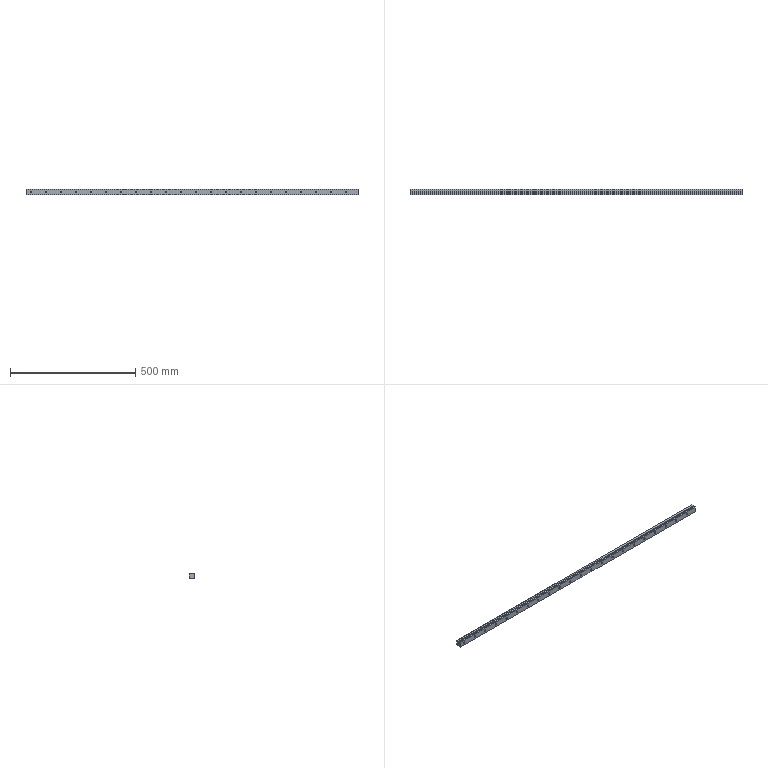Part | NX | features CBORE_HOLE 22, DATUM_CSYS 3, SKETCH 2, EXTRUDE 1, HOLE PACKAGE 1 | 1 solid | 82 faces | box 1328 x 22 x 23 mm | volume 615585 mm3 | cylinder 44 | plane 38 | commonest cylinder face diameters 7 x22 11 x22